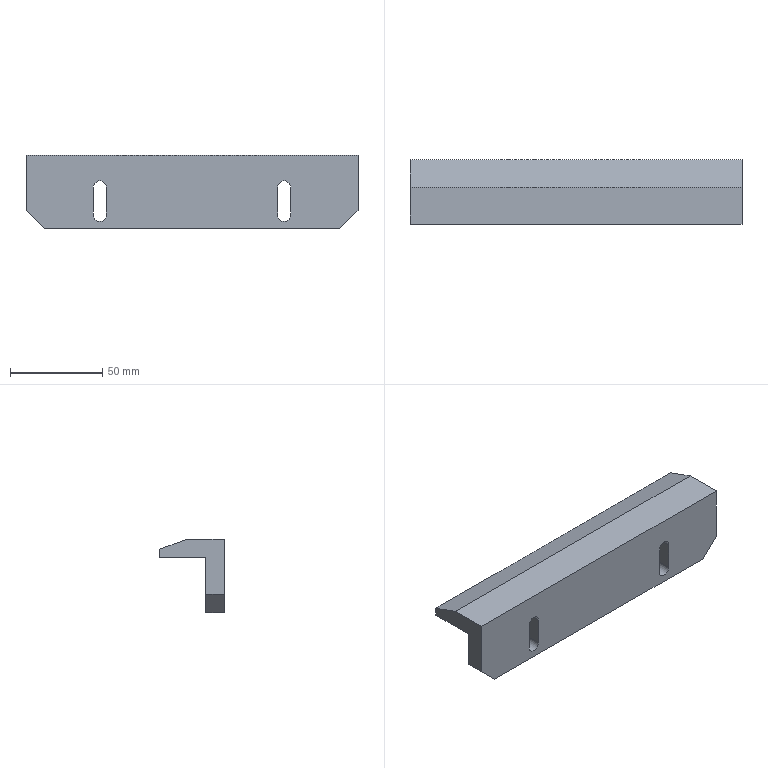Part | SolidWorks | features BaseBody 1 | 1 solid | 19 faces | box 180 x 35 x 40 mm | volume 105760 mm3 | plane 15 | cylinder 4 | commonest cylinder face diameters 7 x4
STEP:
#1=CARTESIAN_POINT('',(-90.,10.,-5.));
#2=VERTEX_POINT('',#1);
#3=CARTESIAN_POINT('',(90.,10.,-5.));
#4=VERTEX_POINT('',#3);
#5=CARTESIAN_POINT('',(90.,10.,-5.));
#6=DIRECTION('',(1.,0.,0.));
#7=VECTOR('',#6,1000.);
#8=LINE('',#5,#7);
#9=EDGE_CURVE('',#2,#4,#8,.T.);
#10=ORIENTED_EDGE('',*,*,#9,.F.);
#11=CARTESIAN_POINT('',(-90.,35.,-5.));
#12=VERTEX_POINT('',#11);
#13=CARTESIAN_POINT('',(-90.,35.,-5.));
#14=DIRECTION('',(0.,-1.,0.));
#15=VECTOR('',#14,1000.);
#16=LINE('',#13,#15);
#17=EDGE_CURVE('',#12,#2,#16,.T.);
#18=ORIENTED_EDGE('',*,*,#17,.F.);
#19=CARTESIAN_POINT('',(90.,35.,-5.));
#20=VERTEX_POINT('',#19);
#21=CARTESIAN_POINT('',(90.,35.,-5.));
#22=DIRECTION('',(-1.,0.,0.));
#23=VECTOR('',#22,1000.);
#24=LINE('',#21,#23);
#25=EDGE_CURVE('',#20,#12,#24,.T.);
#26=ORIENTED_EDGE('',*,*,#25,.F.);
#27=CARTESIAN_POINT('',(90.,35.,-5.));
#28=DIRECTION('',(0.,-1.,0.));
#29=VECTOR('',#28,1000.);
#30=LINE('',#27,#29);
#31=EDGE_CURVE('',#20,#4,#30,.T.);
#32=ORIENTED_EDGE('',*,*,#31,.T.);
#33=EDGE_LOOP('',(#10,#18,#26,#32));
#34=FACE_OUTER_BOUND('',#33,.T.);
#35=CARTESIAN_POINT('',(90.,35.,-5.));
#36=DIRECTION('',(0.,0.,1.));
#37=DIRECTION('',(1.,0.,0.));
#38=AXIS2_PLACEMENT_3D('',#35,#36,#37);
#39=PLANE('',#38);
#40=ADVANCED_FACE('',(#34),#39,.F.);
#41=CARTESIAN_POINT('',(-90.,10.,-25.));
#42=VERTEX_POINT('',#41);
#43=CARTESIAN_POINT('',(-90.,10.,-35.));
#44=DIRECTION('',(0.,0.,1.));
#45=VECTOR('',#44,1000.);
#46=LINE('',#43,#45);
#47=EDGE_CURVE('',#42,#2,#46,.T.);
#48=ORIENTED_EDGE('',*,*,#47,.F.);
#49=CARTESIAN_POINT('',(-90.,0.,-25.));
#50=VERTEX_POINT('',#49);
#51=CARTESIAN_POINT('',(-90.,35.,-25.));
#52=DIRECTION('',(0.,-1.,0.));
#53=VECTOR('',#52,1000.);
#54=LINE('',#51,#53);
#55=EDGE_CURVE('',#42,#50,#54,.T.);
#56=ORIENTED_EDGE('',*,*,#55,.T.);
#57=CARTESIAN_POINT('',(-90.,0.,5.));
#58=VERTEX_POINT('',#57);
#59=CARTESIAN_POINT('',(-90.,0.,5.));
#60=DIRECTION('',(0.,0.,1.));
#61=VECTOR('',#60,1000.);
#62=LINE('',#59,#61);
#63=EDGE_CURVE('',#50,#58,#62,.T.);
#64=ORIENTED_EDGE('',*,*,#63,.T.);
#65=CARTESIAN_POINT('',(-90.,20.,5.));
#66=VERTEX_POINT('',#65);
#67=CARTESIAN_POINT('',(-90.,35.,5.));
#68=DIRECTION('',(0.,-1.,0.));
#69=VECTOR('',#68,1000.);
#70=LINE('',#67,#69);
#71=EDGE_CURVE('',#66,#58,#70,.T.);
#72=ORIENTED_EDGE('',*,*,#71,.F.);
#73=CARTESIAN_POINT('',(-90.,35.,-0.4596));
#74=VERTEX_POINT('',#73);
#75=CARTESIAN_POINT('',(-90.,35.,-0.4596));
#76=DIRECTION('',(0.,0.9397,-0.342));
#77=VECTOR('',#76,1000.);
#78=LINE('',#75,#77);
#79=EDGE_CURVE('',#66,#74,#78,.T.);
#80=ORIENTED_EDGE('',*,*,#79,.T.);
#81=CARTESIAN_POINT('',(-90.,35.,5.));
#82=DIRECTION('',(0.,0.,1.));
#83=VECTOR('',#82,1000.);
#84=LINE('',#81,#83);
#85=EDGE_CURVE('',#12,#74,#84,.T.);
#86=ORIENTED_EDGE('',*,*,#85,.F.);
#87=ORIENTED_EDGE('',*,*,#17,.T.);
#88=EDGE_LOOP('',(#48,#56,#64,#72,#80,#86,#87));
#89=FACE_OUTER_BOUND('',#88,.T.);
#90=CARTESIAN_POINT('',(-90.,35.,5.));
#91=DIRECTION('',(1.,0.,0.));
#92=DIRECTION('',(0.,0.,-1.));
#93=AXIS2_PLACEMENT_3D('',#90,#91,#92);
#94=PLANE('',#93);
#95=ADVANCED_FACE('',(#89),#94,.F.);
#96=CARTESIAN_POINT('',(90.,20.,5.));
#97=VERTEX_POINT('',#96);
#98=CARTESIAN_POINT('',(90.,0.,5.));
#99=VERTEX_POINT('',#98);
#100=CARTESIAN_POINT('',(90.,35.,5.));
#101=DIRECTION('',(0.,-1.,0.));
#102=VECTOR('',#101,1000.);
#103=LINE('',#100,#102);
#104=EDGE_CURVE('',#97,#99,#103,.T.);
#105=ORIENTED_EDGE('',*,*,#104,.F.);
#106=CARTESIAN_POINT('',(-90.,20.,5.));
#107=DIRECTION('',(-1.,0.,0.));
#108=VECTOR('',#107,1000.);
#109=LINE('',#106,#108);
#110=EDGE_CURVE('',#97,#66,#109,.T.);
#111=ORIENTED_EDGE('',*,*,#110,.T.);
#112=ORIENTED_EDGE('',*,*,#71,.T.);
#113=CARTESIAN_POINT('',(90.,0.,5.));
#114=DIRECTION('',(1.,0.,0.));
#115=VECTOR('',#114,1000.);
#116=LINE('',#113,#115);
#117=EDGE_CURVE('',#58,#99,#116,.T.);
#118=ORIENTED_EDGE('',*,*,#117,.T.);
#119=EDGE_LOOP('',(#105,#111,#112,#118));
#120=FACE_OUTER_BOUND('',#119,.T.);
#121=CARTESIAN_POINT('',(90.,35.,5.));
#122=DIRECTION('',(0.,0.,-1.));
#123=DIRECTION('',(-1.,0.,0.));
#124=AXIS2_PLACEMENT_3D('',#121,#122,#123);
#125=PLANE('',#124);
#126=ADVANCED_FACE('',(#120),#125,.F.);
#127=CARTESIAN_POINT('',(90.,0.,-25.));
#128=VERTEX_POINT('',#127);
#129=CARTESIAN_POINT('',(90.,0.,5.));
#130=DIRECTION('',(0.,0.,-1.));
#131=VECTOR('',#130,1000.);
#132=LINE('',#129,#131);
#133=EDGE_CURVE('',#99,#128,#132,.T.);
#134=ORIENTED_EDGE('',*,*,#133,.T.);
#135=CARTESIAN_POINT('',(90.,10.,-25.));
#136=VERTEX_POINT('',#135);
#137=CARTESIAN_POINT('',(90.,35.,-25.));
#138=DIRECTION('',(0.,1.,0.));
#139=VECTOR('',#138,1000.);
#140=LINE('',#137,#139);
#141=EDGE_CURVE('',#128,#136,#140,.T.);
#142=ORIENTED_EDGE('',*,*,#141,.T.);
#143=CARTESIAN_POINT('',(90.,10.,-35.));
#144=DIRECTION('',(0.,0.,1.));
#145=VECTOR('',#144,1000.);
#146=LINE('',#143,#145);
#147=EDGE_CURVE('',#136,#4,#146,.T.);
#148=ORIENTED_EDGE('',*,*,#147,.T.);
#149=ORIENTED_EDGE('',*,*,#31,.F.);
#150=CARTESIAN_POINT('',(90.,35.,-0.4596));
#151=VERTEX_POINT('',#150);
#152=CARTESIAN_POINT('',(90.,35.,5.));
#153=DIRECTION('',(0.,0.,-1.));
#154=VECTOR('',#153,1000.);
#155=LINE('',#152,#154);
#156=EDGE_CURVE('',#151,#20,#155,.T.);
#157=ORIENTED_EDGE('',*,*,#156,.F.);
#158=CARTESIAN_POINT('',(90.,35.,-0.4596));
#159=DIRECTION('',(0.,-0.9397,0.342));
#160=VECTOR('',#159,1000.);
#161=LINE('',#158,#160);
#162=EDGE_CURVE('',#151,#97,#161,.T.);
#163=ORIENTED_EDGE('',*,*,#162,.T.);
#164=ORIENTED_EDGE('',*,*,#104,.T.);
#165=EDGE_LOOP('',(#134,#142,#148,#149,#157,#163,#164));
#166=FACE_OUTER_BOUND('',#165,.T.);
#167=CARTESIAN_POINT('',(90.,35.,5.));
#168=DIRECTION('',(-1.,0.,0.));
#169=DIRECTION('',(0.,0.,1.));
#170=AXIS2_PLACEMENT_3D('',#167,#168,#169);
#171=PLANE('',#170);
#172=ADVANCED_FACE('',(#166),#171,.F.);
#173=ORIENTED_EDGE('',*,*,#85,.T.);
#174=CARTESIAN_POINT('',(90.,35.,-0.4596));
#175=DIRECTION('',(1.,0.,0.));
#176=VECTOR('',#175,1000.);
#177=LINE('',#174,#176);
#178=EDGE_CURVE('',#74,#151,#177,.T.);
#179=ORIENTED_EDGE('',*,*,#178,.T.);
#180=ORIENTED_EDGE('',*,*,#156,.T.);
#181=ORIENTED_EDGE('',*,*,#25,.T.);
#182=EDGE_LOOP('',(#173,#179,#180,#181));
#183=FACE_OUTER_BOUND('',#182,.T.);
#184=CARTESIAN_POINT('',(0.,35.,0.));
#185=DIRECTION('',(0.,1.,0.));
#186=DIRECTION('',(0.,0.,1.));
#187=AXIS2_PLACEMENT_3D('',#184,#185,#186);
#188=PLANE('',#187);
#189=ADVANCED_FACE('',(#183),#188,.T.);
#190=CARTESIAN_POINT('',(53.5,0.,-12.5));
#191=VERTEX_POINT('',#190);
#192=CARTESIAN_POINT('',(53.5,0.,-27.5));
#193=VERTEX_POINT('',#192);
#194=CARTESIAN_POINT('',(53.5,0.,0.));
#195=DIRECTION('',(0.,0.,-1.));
#196=VECTOR('',#195,1000.);
#197=LINE('',#194,#196);
#198=EDGE_CURVE('',#191,#193,#197,.T.);
#199=ORIENTED_EDGE('',*,*,#198,.T.);
#200=CARTESIAN_POINT('',(46.5,0.,-27.5));
#201=VERTEX_POINT('',#200);
#202=CARTESIAN_POINT('',(50.,0.,-27.5));
#203=DIRECTION('',(0.,1.,0.));
#204=DIRECTION('',(0.,0.,1.));
#205=AXIS2_PLACEMENT_3D('',#202,#203,#204);
#206=CIRCLE('',#205,3.5);
#207=EDGE_CURVE('',#193,#201,#206,.T.);
#208=ORIENTED_EDGE('',*,*,#207,.T.);
#209=CARTESIAN_POINT('',(46.5,0.,-12.5));
#210=VERTEX_POINT('',#209);
#211=CARTESIAN_POINT('',(46.5,0.,0.));
#212=DIRECTION('',(0.,0.,1.));
#213=VECTOR('',#212,1000.);
#214=LINE('',#211,#213);
#215=EDGE_CURVE('',#201,#210,#214,.T.);
#216=ORIENTED_EDGE('',*,*,#215,.T.);
#217=CARTESIAN_POINT('',(50.,0.,-12.5));
#218=DIRECTION('',(0.,1.,0.));
#219=DIRECTION('',(0.,0.,1.));
#220=AXIS2_PLACEMENT_3D('',#217,#218,#219);
#221=CIRCLE('',#220,3.5);
#222=EDGE_CURVE('',#210,#191,#221,.T.);
#223=ORIENTED_EDGE('',*,*,#222,.T.);
#224=EDGE_LOOP('',(#199,#208,#216,#223));
#225=FACE_BOUND('',#224,.T.);
#226=CARTESIAN_POINT('',(-46.5,0.,-12.5));
#227=VERTEX_POINT('',#226);
#228=CARTESIAN_POINT('',(-46.5,0.,-27.5));
#229=VERTEX_POINT('',#228);
#230=CARTESIAN_POINT('',(-46.5,0.,0.));
#231=DIRECTION('',(0.,0.,-1.));
#232=VECTOR('',#231,1000.);
#233=LINE('',#230,#232);
#234=EDGE_CURVE('',#227,#229,#233,.T.);
#235=ORIENTED_EDGE('',*,*,#234,.T.);
#236=CARTESIAN_POINT('',(-53.5,0.,-27.5));
#237=VERTEX_POINT('',#236);
#238=CARTESIAN_POINT('',(-50.,0.,-27.5));
#239=DIRECTION('',(0.,1.,0.));
#240=DIRECTION('',(0.,0.,1.));
#241=AXIS2_PLACEMENT_3D('',#238,#239,#240);
#242=CIRCLE('',#241,3.5);
#243=EDGE_CURVE('',#229,#237,#242,.T.);
#244=ORIENTED_EDGE('',*,*,#243,.T.);
#245=CARTESIAN_POINT('',(-53.5,0.,-12.5));
#246=VERTEX_POINT('',#245);
#247=CARTESIAN_POINT('',(-53.5,0.,0.));
#248=DIRECTION('',(0.,0.,1.));
#249=VECTOR('',#248,1000.);
#250=LINE('',#247,#249);
#251=EDGE_CURVE('',#237,#246,#250,.T.);
#252=ORIENTED_EDGE('',*,*,#251,.T.);
#253=CARTESIAN_POINT('',(-50.,0.,-12.5));
#254=DIRECTION('',(0.,1.,0.));
#255=DIRECTION('',(0.,0.,1.));
#256=AXIS2_PLACEMENT_3D('',#253,#254,#255);
#257=CIRCLE('',#256,3.5);
#258=EDGE_CURVE('',#246,#227,#257,.T.);
#259=ORIENTED_EDGE('',*,*,#258,.T.);
#260=EDGE_LOOP('',(#235,#244,#252,#259));
#261=FACE_BOUND('',#260,.T.);
#262=ORIENTED_EDGE('',*,*,#63,.F.);
#263=CARTESIAN_POINT('',(-80.,0.,-35.));
#264=VERTEX_POINT('',#263);
#265=CARTESIAN_POINT('',(-80.,0.,-35.));
#266=DIRECTION('',(0.7071,0.,-0.7071));
#267=VECTOR('',#266,1000.);
#268=LINE('',#265,#267);
#269=EDGE_CURVE('',#50,#264,#268,.T.);
#270=ORIENTED_EDGE('',*,*,#269,.T.);
#271=CARTESIAN_POINT('',(80.,0.,-35.));
#272=VERTEX_POINT('',#271);
#273=CARTESIAN_POINT('',(90.,0.,-35.));
#274=DIRECTION('',(-1.,0.,0.));
#275=VECTOR('',#274,1000.);
#276=LINE('',#273,#275);
#277=EDGE_CURVE('',#272,#264,#276,.T.);
#278=ORIENTED_EDGE('',*,*,#277,.F.);
#279=CARTESIAN_POINT('',(80.,0.,-35.));
#280=DIRECTION('',(0.7071,0.,0.7071));
#281=VECTOR('',#280,1000.);
#282=LINE('',#279,#281);
#283=EDGE_CURVE('',#272,#128,#282,.T.);
#284=ORIENTED_EDGE('',*,*,#283,.T.);
#285=ORIENTED_EDGE('',*,*,#133,.F.);
#286=ORIENTED_EDGE('',*,*,#117,.F.);
#287=EDGE_LOOP('',(#262,#270,#278,#284,#285,#286));
#288=FACE_OUTER_BOUND('',#287,.T.);
#289=CARTESIAN_POINT('',(0.,0.,0.));
#290=DIRECTION('',(0.,1.,0.));
#291=DIRECTION('',(0.,0.,1.));
#292=AXIS2_PLACEMENT_3D('',#289,#290,#291);
#293=PLANE('',#292);
#294=ADVANCED_FACE('',(#225,#261,#288),#293,.F.);
#295=ORIENTED_EDGE('',*,*,#79,.F.);
#296=ORIENTED_EDGE('',*,*,#110,.F.);
#297=ORIENTED_EDGE('',*,*,#162,.F.);
#298=ORIENTED_EDGE('',*,*,#178,.F.);
#299=EDGE_LOOP('',(#295,#296,#297,#298));
#300=FACE_OUTER_BOUND('',#299,.T.);
#301=CARTESIAN_POINT('',(0.,35.,-0.4596));
#302=DIRECTION('',(0.,0.342,0.9397));
#303=DIRECTION('',(-1.,0.,0.));
#304=AXIS2_PLACEMENT_3D('',#301,#302,#303);
#305=PLANE('',#304);
#306=ADVANCED_FACE('',(#300),#305,.T.);
#307=CARTESIAN_POINT('',(46.5,10.,-27.5));
#308=VERTEX_POINT('',#307);
#309=CARTESIAN_POINT('',(46.5,10.,-12.5));
#310=VERTEX_POINT('',#309);
#311=CARTESIAN_POINT('',(46.5,10.,-27.5));
#312=DIRECTION('',(0.,0.,1.));
#313=VECTOR('',#312,1000.);
#314=LINE('',#311,#313);
#315=EDGE_CURVE('',#308,#310,#314,.T.);
#316=ORIENTED_EDGE('',*,*,#315,.F.);
#317=CARTESIAN_POINT('',(53.5,10.,-27.5));
#318=VERTEX_POINT('',#317);
#319=CARTESIAN_POINT('',(50.,10.,-27.5));
#320=DIRECTION('',(0.,1.,0.));
#321=DIRECTION('',(1.,0.,0.));
#322=AXIS2_PLACEMENT_3D('',#319,#320,#321);
#323=CIRCLE('',#322,3.5);
#324=EDGE_CURVE('',#318,#308,#323,.T.);
#325=ORIENTED_EDGE('',*,*,#324,.F.);
#326=CARTESIAN_POINT('',(53.5,10.,-12.5));
#327=VERTEX_POINT('',#326);
#328=CARTESIAN_POINT('',(53.5,10.,-27.5));
#329=DIRECTION('',(0.,0.,-1.));
#330=VECTOR('',#329,1000.);
#331=LINE('',#328,#330);
#332=EDGE_CURVE('',#327,#318,#331,.T.);
#333=ORIENTED_EDGE('',*,*,#332,.F.);
#334=CARTESIAN_POINT('',(50.,10.,-12.5));
#335=DIRECTION('',(0.,1.,0.));
#336=DIRECTION('',(1.,0.,0.));
#337=AXIS2_PLACEMENT_3D('',#334,#335,#336);
#338=CIRCLE('',#337,3.5);
#339=EDGE_CURVE('',#310,#327,#338,.T.);
#340=ORIENTED_EDGE('',*,*,#339,.F.);
#341=EDGE_LOOP('',(#316,#325,#333,#340));
#342=FACE_BOUND('',#341,.T.);
#343=CARTESIAN_POINT('',(-53.5,10.,-27.5));
#344=VERTEX_POINT('',#343);
#345=CARTESIAN_POINT('',(-53.5,10.,-12.5));
#346=VERTEX_POINT('',#345);
#347=CARTESIAN_POINT('',(-53.5,10.,-27.5));
#348=DIRECTION('',(0.,0.,1.));
#349=VECTOR('',#348,1000.);
#350=LINE('',#347,#349);
#351=EDGE_CURVE('',#344,#346,#350,.T.);
#352=ORIENTED_EDGE('',*,*,#351,.F.);
#353=CARTESIAN_POINT('',(-46.5,10.,-27.5));
#354=VERTEX_POINT('',#353);
#355=CARTESIAN_POINT('',(-50.,10.,-27.5));
#356=DIRECTION('',(0.,1.,0.));
#357=DIRECTION('',(-1.,0.,0.));
#358=AXIS2_PLACEMENT_3D('',#355,#356,#357);
#359=CIRCLE('',#358,3.5);
#360=EDGE_CURVE('',#354,#344,#359,.T.);
#361=ORIENTED_EDGE('',*,*,#360,.F.);
#362=CARTESIAN_POINT('',(-46.5,10.,-12.5));
#363=VERTEX_POINT('',#362);
#364=CARTESIAN_POINT('',(-46.5,10.,-27.5));
#365=DIRECTION('',(0.,0.,-1.));
#366=VECTOR('',#365,1000.);
#367=LINE('',#364,#366);
#368=EDGE_CURVE('',#363,#354,#367,.T.);
#369=ORIENTED_EDGE('',*,*,#368,.F.);
#370=CARTESIAN_POINT('',(-50.,10.,-12.5));
#371=DIRECTION('',(0.,1.,0.));
#372=DIRECTION('',(-1.,0.,0.));
#373=AXIS2_PLACEMENT_3D('',#370,#371,#372);
#374=CIRCLE('',#373,3.5);
#375=EDGE_CURVE('',#346,#363,#374,.T.);
#376=ORIENTED_EDGE('',*,*,#375,.F.);
#377=EDGE_LOOP('',(#352,#361,#369,#376));
#378=FACE_BOUND('',#377,.T.);
#379=CARTESIAN_POINT('',(-80.,10.,-35.));
#380=VERTEX_POINT('',#379);
#381=CARTESIAN_POINT('',(80.,10.,-35.));
#382=VERTEX_POINT('',#381);
#383=CARTESIAN_POINT('',(90.,10.,-35.));
#384=DIRECTION('',(1.,0.,0.));
#385=VECTOR('',#384,1000.);
#386=LINE('',#383,#385);
#387=EDGE_CURVE('',#380,#382,#386,.T.);
#388=ORIENTED_EDGE('',*,*,#387,.F.);
#389=CARTESIAN_POINT('',(-80.,10.,-35.));
#390=DIRECTION('',(-0.7071,0.,0.7071));
#391=VECTOR('',#390,1000.);
#392=LINE('',#389,#391);
#393=EDGE_CURVE('',#380,#42,#392,.T.);
#394=ORIENTED_EDGE('',*,*,#393,.T.);
#395=ORIENTED_EDGE('',*,*,#47,.T.);
#396=ORIENTED_EDGE('',*,*,#9,.T.);
#397=ORIENTED_EDGE('',*,*,#147,.F.);
#398=CARTESIAN_POINT('',(80.,10.,-35.));
#399=DIRECTION('',(-0.7071,0.,-0.7071));
#400=VECTOR('',#399,1000.);
#401=LINE('',#398,#400);
#402=EDGE_CURVE('',#136,#382,#401,.T.);
#403=ORIENTED_EDGE('',*,*,#402,.T.);
#404=EDGE_LOOP('',(#388,#394,#395,#396,#397,#403));
#405=FACE_OUTER_BOUND('',#404,.T.);
#406=CARTESIAN_POINT('',(90.,10.,-35.));
#407=DIRECTION('',(0.,-1.,0.));
#408=DIRECTION('',(1.,0.,0.));
#409=AXIS2_PLACEMENT_3D('',#406,#407,#408);
#410=PLANE('',#409);
#411=ADVANCED_FACE('',(#342,#378,#405),#410,.F.);
#412=ORIENTED_EDGE('',*,*,#277,.T.);
#413=CARTESIAN_POINT('',(-80.,0.,-35.));
#414=DIRECTION('',(0.,1.,0.));
#415=VECTOR('',#414,1000.);
#416=LINE('',#413,#415);
#417=EDGE_CURVE('',#264,#380,#416,.T.);
#418=ORIENTED_EDGE('',*,*,#417,.T.);
#419=ORIENTED_EDGE('',*,*,#387,.T.);
#420=CARTESIAN_POINT('',(80.,0.,-35.));
#421=DIRECTION('',(0.,-1.,0.));
#422=VECTOR('',#421,1000.);
#423=LINE('',#420,#422);
#424=EDGE_CURVE('',#382,#272,#423,.T.);
#425=ORIENTED_EDGE('',*,*,#424,.T.);
#426=EDGE_LOOP('',(#412,#418,#419,#425));
#427=FACE_OUTER_BOUND('',#426,.T.);
#428=CARTESIAN_POINT('',(0.,0.,-35.));
#429=DIRECTION('',(0.,0.,1.));
#430=DIRECTION('',(1.,0.,0.));
#431=AXIS2_PLACEMENT_3D('',#428,#429,#430);
#432=PLANE('',#431);
#433=ADVANCED_FACE('',(#427),#432,.F.);
#434=ORIENTED_EDGE('',*,*,#269,.F.);
#435=ORIENTED_EDGE('',*,*,#55,.F.);
#436=ORIENTED_EDGE('',*,*,#393,.F.);
#437=ORIENTED_EDGE('',*,*,#417,.F.);
#438=EDGE_LOOP('',(#434,#435,#436,#437));
#439=FACE_OUTER_BOUND('',#438,.T.);
#440=CARTESIAN_POINT('',(-80.,0.,-35.));
#441=DIRECTION('',(0.7071,0.,0.7071));
#442=DIRECTION('',(0.,1.,0.));
#443=AXIS2_PLACEMENT_3D('',#440,#441,#442);
#444=PLANE('',#443);
#445=ADVANCED_FACE('',(#439),#444,.F.);
#446=ORIENTED_EDGE('',*,*,#402,.F.);
#447=ORIENTED_EDGE('',*,*,#141,.F.);
#448=ORIENTED_EDGE('',*,*,#283,.F.);
#449=ORIENTED_EDGE('',*,*,#424,.F.);
#450=EDGE_LOOP('',(#446,#447,#448,#449));
#451=FACE_OUTER_BOUND('',#450,.T.);
#452=CARTESIAN_POINT('',(80.,0.,-35.));
#453=DIRECTION('',(-0.7071,0.,0.7071));
#454=DIRECTION('',(0.,-1.,0.));
#455=AXIS2_PLACEMENT_3D('',#452,#453,#454);
#456=PLANE('',#455);
#457=ADVANCED_FACE('',(#451),#456,.F.);
#458=CARTESIAN_POINT('',(-46.5,-30.,-27.5));
#459=DIRECTION('',(0.,1.,0.));
#460=VECTOR('',#459,1000.);
#461=LINE('',#458,#460);
#462=EDGE_CURVE('',#229,#354,#461,.T.);
#463=ORIENTED_EDGE('',*,*,#462,.T.);
#464=ORIENTED_EDGE('',*,*,#360,.T.);
#465=CARTESIAN_POINT('',(-53.5,-30.,-27.5));
#466=DIRECTION('',(0.,1.,0.));
#467=VECTOR('',#466,1000.);
#468=LINE('',#465,#467);
#469=EDGE_CURVE('',#237,#344,#468,.T.);
#470=ORIENTED_EDGE('',*,*,#469,.F.);
#471=ORIENTED_EDGE('',*,*,#243,.F.);
#472=EDGE_LOOP('',(#463,#464,#470,#471));
#473=FACE_OUTER_BOUND('',#472,.T.);
#474=CARTESIAN_POINT('',(-50.,-30.,-27.5));
#475=DIRECTION('',(0.,1.,0.));
#476=DIRECTION('',(-1.,0.,0.));
#477=AXIS2_PLACEMENT_3D('',#474,#475,#476);
#478=CYLINDRICAL_SURFACE('',#477,3.5);
#479=ADVANCED_FACE('',(#473),#478,.F.);
#480=CARTESIAN_POINT('',(-46.5,-30.,-12.5));
#481=DIRECTION('',(0.,1.,0.));
#482=VECTOR('',#481,1000.);
#483=LINE('',#480,#482);
#484=EDGE_CURVE('',#227,#363,#483,.T.);
#485=ORIENTED_EDGE('',*,*,#484,.T.);
#486=ORIENTED_EDGE('',*,*,#368,.T.);
#487=ORIENTED_EDGE('',*,*,#462,.F.);
#488=ORIENTED_EDGE('',*,*,#234,.F.);
#489=EDGE_LOOP('',(#485,#486,#487,#488));
#490=FACE_OUTER_BOUND('',#489,.T.);
#491=CARTESIAN_POINT('',(-46.5,-30.,-27.5));
#492=DIRECTION('',(1.,0.,0.));
#493=DIRECTION('',(0.,0.,-1.));
#494=AXIS2_PLACEMENT_3D('',#491,#492,#493);
#495=PLANE('',#494);
#496=ADVANCED_FACE('',(#490),#495,.F.);
#497=CARTESIAN_POINT('',(-53.5,-30.,-12.5));
#498=DIRECTION('',(0.,1.,0.));
#499=VECTOR('',#498,1000.);
#500=LINE('',#497,#499);
#501=EDGE_CURVE('',#246,#346,#500,.T.);
#502=ORIENTED_EDGE('',*,*,#501,.T.);
#503=ORIENTED_EDGE('',*,*,#375,.T.);
#504=ORIENTED_EDGE('',*,*,#484,.F.);
#505=ORIENTED_EDGE('',*,*,#258,.F.);
#506=EDGE_LOOP('',(#502,#503,#504,#505));
#507=FACE_OUTER_BOUND('',#506,.T.);
#508=CARTESIAN_POINT('',(-50.,-30.,-12.5));
#509=DIRECTION('',(0.,1.,0.));
#510=DIRECTION('',(-1.,0.,0.));
#511=AXIS2_PLACEMENT_3D('',#508,#509,#510);
#512=CYLINDRICAL_SURFACE('',#511,3.5);
#513=ADVANCED_FACE('',(#507),#512,.F.);
#514=ORIENTED_EDGE('',*,*,#469,.T.);
#515=ORIENTED_EDGE('',*,*,#351,.T.);
#516=ORIENTED_EDGE('',*,*,#501,.F.);
#517=ORIENTED_EDGE('',*,*,#251,.F.);
#518=EDGE_LOOP('',(#514,#515,#516,#517));
#519=FACE_OUTER_BOUND('',#518,.T.);
#520=CARTESIAN_POINT('',(-53.5,-30.,-27.5));
#521=DIRECTION('',(-1.,0.,0.));
#522=DIRECTION('',(0.,0.,1.));
#523=AXIS2_PLACEMENT_3D('',#520,#521,#522);
#524=PLANE('',#523);
#525=ADVANCED_FACE('',(#519),#524,.F.);
#526=CARTESIAN_POINT('',(53.5,-30.,-27.5));
#527=DIRECTION('',(0.,1.,0.));
#528=VECTOR('',#527,1000.);
#529=LINE('',#526,#528);
#530=EDGE_CURVE('',#193,#318,#529,.T.);
#531=ORIENTED_EDGE('',*,*,#530,.T.);
#532=ORIENTED_EDGE('',*,*,#324,.T.);
#533=CARTESIAN_POINT('',(46.5,-30.,-27.5));
#534=DIRECTION('',(0.,1.,0.));
#535=VECTOR('',#534,1000.);
#536=LINE('',#533,#535);
#537=EDGE_CURVE('',#201,#308,#536,.T.);
#538=ORIENTED_EDGE('',*,*,#537,.F.);
#539=ORIENTED_EDGE('',*,*,#207,.F.);
#540=EDGE_LOOP('',(#531,#532,#538,#539));
#541=FACE_OUTER_BOUND('',#540,.T.);
#542=CARTESIAN_POINT('',(50.,-30.,-27.5));
#543=DIRECTION('',(0.,1.,0.));
#544=DIRECTION('',(-1.,0.,0.));
#545=AXIS2_PLACEMENT_3D('',#542,#543,#544);
#546=CYLINDRICAL_SURFACE('',#545,3.5);
#547=ADVANCED_FACE('',(#541),#546,.F.);
#548=CARTESIAN_POINT('',(53.5,-30.,-12.5));
#549=DIRECTION('',(0.,1.,0.));
#550=VECTOR('',#549,1000.);
#551=LINE('',#548,#550);
#552=EDGE_CURVE('',#191,#327,#551,.T.);
#553=ORIENTED_EDGE('',*,*,#552,.T.);
#554=ORIENTED_EDGE('',*,*,#332,.T.);
#555=ORIENTED_EDGE('',*,*,#530,.F.);
#556=ORIENTED_EDGE('',*,*,#198,.F.);
#557=EDGE_LOOP('',(#553,#554,#555,#556));
#558=FACE_OUTER_BOUND('',#557,.T.);
#559=CARTESIAN_POINT('',(53.5,-30.,-27.5));
#560=DIRECTION('',(1.,0.,0.));
#561=DIRECTION('',(0.,0.,-1.));
#562=AXIS2_PLACEMENT_3D('',#559,#560,#561);
#563=PLANE('',#562);
#564=ADVANCED_FACE('',(#558),#563,.F.);
#565=CARTESIAN_POINT('',(46.5,-30.,-12.5));
#566=DIRECTION('',(0.,1.,0.));
#567=VECTOR('',#566,1000.);
#568=LINE('',#565,#567);
#569=EDGE_CURVE('',#210,#310,#568,.T.);
#570=ORIENTED_EDGE('',*,*,#569,.T.);
#571=ORIENTED_EDGE('',*,*,#339,.T.);
#572=ORIENTED_EDGE('',*,*,#552,.F.);
#573=ORIENTED_EDGE('',*,*,#222,.F.);
#574=EDGE_LOOP('',(#570,#571,#572,#573));
#575=FACE_OUTER_BOUND('',#574,.T.);
#576=CARTESIAN_POINT('',(50.,-30.,-12.5));
#577=DIRECTION('',(0.,1.,0.));
#578=DIRECTION('',(-1.,0.,0.));
#579=AXIS2_PLACEMENT_3D('',#576,#577,#578);
#580=CYLINDRICAL_SURFACE('',#579,3.5);
#581=ADVANCED_FACE('',(#575),#580,.F.);
#582=ORIENTED_EDGE('',*,*,#537,.T.);
#583=ORIENTED_EDGE('',*,*,#315,.T.);
#584=ORIENTED_EDGE('',*,*,#569,.F.);
#585=ORIENTED_EDGE('',*,*,#215,.F.);
#586=EDGE_LOOP('',(#582,#583,#584,#585));
#587=FACE_OUTER_BOUND('',#586,.T.);
#588=CARTESIAN_POINT('',(46.5,-30.,-27.5));
#589=DIRECTION('',(-1.,0.,0.));
#590=DIRECTION('',(0.,0.,1.));
#591=AXIS2_PLACEMENT_3D('',#588,#589,#590);
#592=PLANE('',#591);
#593=ADVANCED_FACE('',(#587),#592,.F.);
#594=CLOSED_SHELL('',(#40,#95,#126,#172,#189,#294,#306,#411,#433,#445,#457,#479,#496,#513,#525,#547,#564,#581,#593));
#595=MANIFOLD_SOLID_BREP('',#594);
#596=CARTESIAN_POINT('',(0.,0.,0.));
#597=DIRECTION('',(0.,0.,1.));
#598=DIRECTION('',(1.,0.,0.));
#599=AXIS2_PLACEMENT_3D('',#596,#597,#598);
#600=(LENGTH_UNIT()NAMED_UNIT(*)SI_UNIT(.MILLI.,.METRE.));
#601=UNCERTAINTY_MEASURE_WITH_UNIT(LENGTH_MEASURE(0.00001),#600,'','');
#602=(NAMED_UNIT(*)PLANE_ANGLE_UNIT()SI_UNIT($,.RADIAN.));
#603=(NAMED_UNIT(*)SI_UNIT($,.STERADIAN.)SOLID_ANGLE_UNIT());
#604=(GEOMETRIC_REPRESENTATION_CONTEXT(3)GLOBAL_UNCERTAINTY_ASSIGNED_CONTEXT((#601))GLOBAL_UNIT_ASSIGNED_CONTEXT((#600,#602,#603))REPRESENTATION_CONTEXT('',''));
#605=ADVANCED_BREP_SHAPE_REPRESENTATION('',(#595,#599),#604);